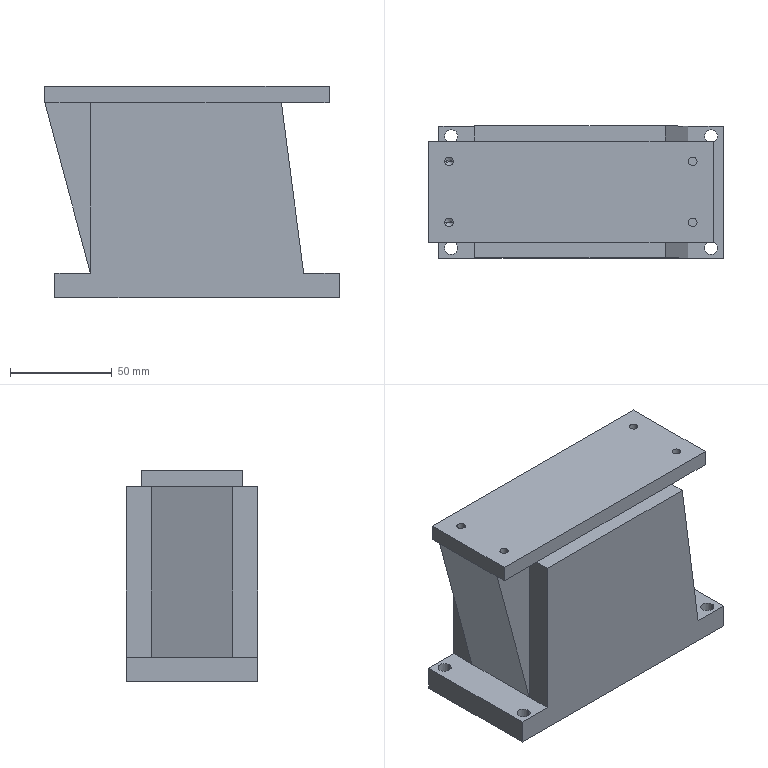Part | STEP file | Direct vibration | 1 solid | 43 faces | box 145 x 65 x 104 mm | volume 744100 mm3 | plane 23 | cylinder 16 | cone 4 | commonest cylinder face diameters 4.2 x8 6.5 x8